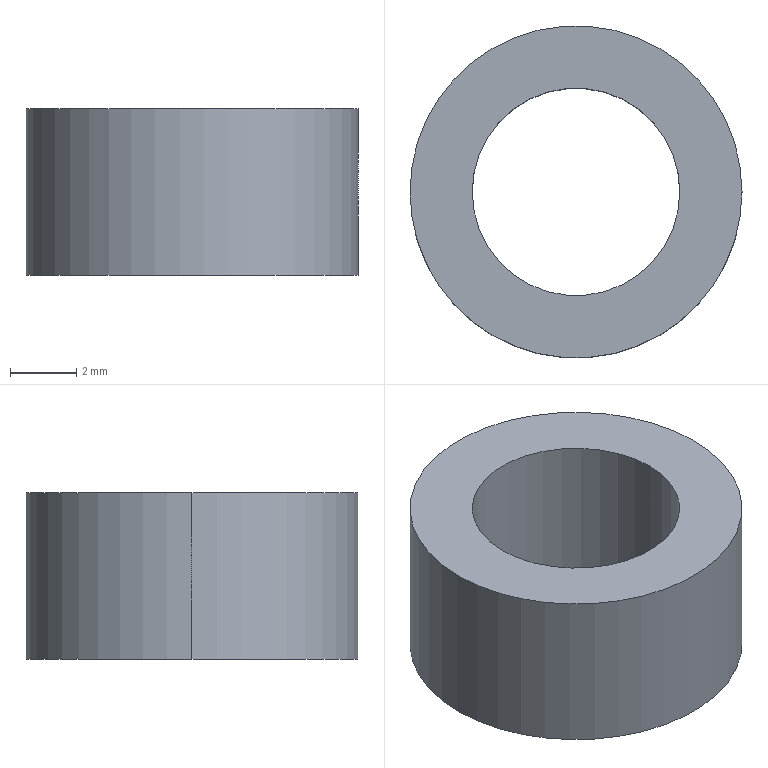Part | SolidWorks | features Extrusion 1 | 1 solid | 6 faces | box 10 x 10 x 5 mm | volume 239.301 mm3 | cylinder 4 | plane 2 | commonest cylinder face diameters 6.25 x2 10 x2
STEP:
#1=CARTESIAN_POINT('',(-0.123,0.,0.1969));
#2=VERTEX_POINT('',#1);
#3=CARTESIAN_POINT('',(0.123,0.,0.1969));
#4=VERTEX_POINT('',#3);
#5=CARTESIAN_POINT('',(0.,0.,0.1969));
#6=DIRECTION('',(0.,0.,1.));
#7=DIRECTION('',(1.,0.,0.));
#8=AXIS2_PLACEMENT_3D('',#5,#6,#7);
#9=CIRCLE('',#8,0.123);
#10=EDGE_CURVE('',#2,#4,#9,.T.);
#11=ORIENTED_EDGE('',*,*,#10,.T.);
#12=CARTESIAN_POINT('',(0.123,0.,0.));
#13=VERTEX_POINT('',#12);
#14=CARTESIAN_POINT('',(0.123,0.,0.1969));
#15=DIRECTION('',(0.,0.,-1.));
#16=VECTOR('',#15,39.37);
#17=LINE('',#14,#16);
#18=EDGE_CURVE('',#4,#13,#17,.T.);
#19=ORIENTED_EDGE('',*,*,#18,.T.);
#20=CARTESIAN_POINT('',(-0.123,0.,0.));
#21=VERTEX_POINT('',#20);
#22=CARTESIAN_POINT('',(0.,0.,0.));
#23=DIRECTION('',(0.,0.,1.));
#24=DIRECTION('',(1.,0.,0.));
#25=AXIS2_PLACEMENT_3D('',#22,#23,#24);
#26=CIRCLE('',#25,0.123);
#27=EDGE_CURVE('',#21,#13,#26,.T.);
#28=ORIENTED_EDGE('',*,*,#27,.F.);
#29=CARTESIAN_POINT('',(-0.123,0.,0.1969));
#30=DIRECTION('',(0.,0.,-1.));
#31=VECTOR('',#30,39.37);
#32=LINE('',#29,#31);
#33=EDGE_CURVE('',#2,#21,#32,.T.);
#34=ORIENTED_EDGE('',*,*,#33,.F.);
#35=EDGE_LOOP('',(#11,#19,#28,#34));
#36=FACE_OUTER_BOUND('',#35,.T.);
#37=CARTESIAN_POINT('',(0.,0.,0.1969));
#38=DIRECTION('',(0.,0.,-1.));
#39=DIRECTION('',(-1.,0.,0.));
#40=AXIS2_PLACEMENT_3D('',#37,#38,#39);
#41=CYLINDRICAL_SURFACE('',#40,0.123);
#42=ADVANCED_FACE('',(#36),#41,.F.);
#43=CARTESIAN_POINT('',(0.1969,0.,0.1969));
#44=VERTEX_POINT('',#43);
#45=CARTESIAN_POINT('',(-0.1969,0.,0.1969));
#46=VERTEX_POINT('',#45);
#47=CARTESIAN_POINT('',(0.,0.,0.1969));
#48=DIRECTION('',(0.,0.,1.));
#49=DIRECTION('',(1.,0.,0.));
#50=AXIS2_PLACEMENT_3D('',#47,#48,#49);
#51=CIRCLE('',#50,0.1969);
#52=EDGE_CURVE('',#44,#46,#51,.T.);
#53=ORIENTED_EDGE('',*,*,#52,.F.);
#54=CARTESIAN_POINT('',(0.1969,0.,0.));
#55=VERTEX_POINT('',#54);
#56=CARTESIAN_POINT('',(0.1969,0.,0.1969));
#57=DIRECTION('',(0.,0.,-1.));
#58=VECTOR('',#57,39.37);
#59=LINE('',#56,#58);
#60=EDGE_CURVE('',#44,#55,#59,.T.);
#61=ORIENTED_EDGE('',*,*,#60,.T.);
#62=CARTESIAN_POINT('',(-0.1969,0.,0.));
#63=VERTEX_POINT('',#62);
#64=CARTESIAN_POINT('',(0.,0.,0.));
#65=DIRECTION('',(0.,0.,1.));
#66=DIRECTION('',(1.,0.,0.));
#67=AXIS2_PLACEMENT_3D('',#64,#65,#66);
#68=CIRCLE('',#67,0.1969);
#69=EDGE_CURVE('',#55,#63,#68,.T.);
#70=ORIENTED_EDGE('',*,*,#69,.T.);
#71=CARTESIAN_POINT('',(-0.1969,0.,0.1969));
#72=DIRECTION('',(0.,0.,-1.));
#73=VECTOR('',#72,39.37);
#74=LINE('',#71,#73);
#75=EDGE_CURVE('',#46,#63,#74,.T.);
#76=ORIENTED_EDGE('',*,*,#75,.F.);
#77=EDGE_LOOP('',(#53,#61,#70,#76));
#78=FACE_OUTER_BOUND('',#77,.T.);
#79=CARTESIAN_POINT('',(0.,0.,0.1969));
#80=DIRECTION('',(0.,0.,-1.));
#81=DIRECTION('',(-1.,0.,0.));
#82=AXIS2_PLACEMENT_3D('',#79,#80,#81);
#83=CYLINDRICAL_SURFACE('',#82,0.1969);
#84=ADVANCED_FACE('',(#78),#83,.T.);
#85=CARTESIAN_POINT('',(0.,0.,0.1969));
#86=DIRECTION('',(0.,0.,1.));
#87=DIRECTION('',(1.,0.,0.));
#88=AXIS2_PLACEMENT_3D('',#85,#86,#87);
#89=CIRCLE('',#88,0.1969);
#90=EDGE_CURVE('',#46,#44,#89,.T.);
#91=ORIENTED_EDGE('',*,*,#90,.T.);
#92=ORIENTED_EDGE('',*,*,#52,.T.);
#93=EDGE_LOOP('',(#91,#92));
#94=FACE_OUTER_BOUND('',#93,.T.);
#95=ORIENTED_EDGE('',*,*,#10,.F.);
#96=CARTESIAN_POINT('',(0.,0.,0.1969));
#97=DIRECTION('',(0.,0.,1.));
#98=DIRECTION('',(1.,0.,0.));
#99=AXIS2_PLACEMENT_3D('',#96,#97,#98);
#100=CIRCLE('',#99,0.123);
#101=EDGE_CURVE('',#4,#2,#100,.T.);
#102=ORIENTED_EDGE('',*,*,#101,.F.);
#103=EDGE_LOOP('',(#95,#102));
#104=FACE_BOUND('',#103,.T.);
#105=CARTESIAN_POINT('',(0.,0.,0.1969));
#106=DIRECTION('',(0.,0.,1.));
#107=DIRECTION('',(1.,0.,0.));
#108=AXIS2_PLACEMENT_3D('',#105,#106,#107);
#109=PLANE('',#108);
#110=ADVANCED_FACE('',(#94,#104),#109,.T.);
#111=CARTESIAN_POINT('',(0.,0.,0.));
#112=DIRECTION('',(0.,0.,1.));
#113=DIRECTION('',(1.,0.,0.));
#114=AXIS2_PLACEMENT_3D('',#111,#112,#113);
#115=CIRCLE('',#114,0.1969);
#116=EDGE_CURVE('',#63,#55,#115,.T.);
#117=ORIENTED_EDGE('',*,*,#116,.F.);
#118=ORIENTED_EDGE('',*,*,#69,.F.);
#119=EDGE_LOOP('',(#117,#118));
#120=FACE_OUTER_BOUND('',#119,.T.);
#121=ORIENTED_EDGE('',*,*,#27,.T.);
#122=CARTESIAN_POINT('',(0.,0.,0.));
#123=DIRECTION('',(0.,0.,1.));
#124=DIRECTION('',(1.,0.,0.));
#125=AXIS2_PLACEMENT_3D('',#122,#123,#124);
#126=CIRCLE('',#125,0.123);
#127=EDGE_CURVE('',#13,#21,#126,.T.);
#128=ORIENTED_EDGE('',*,*,#127,.T.);
#129=EDGE_LOOP('',(#121,#128));
#130=FACE_BOUND('',#129,.T.);
#131=CARTESIAN_POINT('',(0.,0.,0.));
#132=DIRECTION('',(0.,0.,1.));
#133=DIRECTION('',(1.,0.,0.));
#134=AXIS2_PLACEMENT_3D('',#131,#132,#133);
#135=PLANE('',#134);
#136=ADVANCED_FACE('',(#120,#130),#135,.F.);
#137=ORIENTED_EDGE('',*,*,#60,.F.);
#138=ORIENTED_EDGE('',*,*,#90,.F.);
#139=ORIENTED_EDGE('',*,*,#75,.T.);
#140=ORIENTED_EDGE('',*,*,#116,.T.);
#141=EDGE_LOOP('',(#137,#138,#139,#140));
#142=FACE_OUTER_BOUND('',#141,.T.);
#143=CARTESIAN_POINT('',(0.,0.,0.1969));
#144=DIRECTION('',(0.,0.,-1.));
#145=DIRECTION('',(-1.,0.,0.));
#146=AXIS2_PLACEMENT_3D('',#143,#144,#145);
#147=CYLINDRICAL_SURFACE('',#146,0.1969);
#148=ADVANCED_FACE('',(#142),#147,.T.);
#149=ORIENTED_EDGE('',*,*,#18,.F.);
#150=ORIENTED_EDGE('',*,*,#101,.T.);
#151=ORIENTED_EDGE('',*,*,#33,.T.);
#152=ORIENTED_EDGE('',*,*,#127,.F.);
#153=EDGE_LOOP('',(#149,#150,#151,#152));
#154=FACE_OUTER_BOUND('',#153,.T.);
#155=CARTESIAN_POINT('',(0.,0.,0.1969));
#156=DIRECTION('',(0.,0.,-1.));
#157=DIRECTION('',(-1.,0.,0.));
#158=AXIS2_PLACEMENT_3D('',#155,#156,#157);
#159=CYLINDRICAL_SURFACE('',#158,0.123);
#160=ADVANCED_FACE('',(#154),#159,.F.);
#161=CLOSED_SHELL('',(#42,#84,#110,#136,#148,#160));
#162=MANIFOLD_SOLID_BREP('',#161);
#163=CARTESIAN_POINT('',(0.,0.,0.));
#164=DIRECTION('',(0.,0.,1.));
#165=DIRECTION('',(1.,0.,0.));
#166=AXIS2_PLACEMENT_3D('',#163,#164,#165);
#167=(LENGTH_UNIT()NAMED_UNIT(*)SI_UNIT($,.METRE.));
#168=LENGTH_MEASURE_WITH_UNIT(LENGTH_MEASURE(0.0254),#167);
#169=DIMENSIONAL_EXPONENTS(1.,0.,0.,0.,0.,0.,0.);
#170=(CONVERSION_BASED_UNIT('INCH',#168)LENGTH_UNIT()NAMED_UNIT(#169));
#171=UNCERTAINTY_MEASURE_WITH_UNIT(LENGTH_MEASURE(0.00001),#170,'','');
#172=(NAMED_UNIT(*)PLANE_ANGLE_UNIT()SI_UNIT($,.RADIAN.));
#173=(NAMED_UNIT(*)SI_UNIT($,.STERADIAN.)SOLID_ANGLE_UNIT());
#174=(GEOMETRIC_REPRESENTATION_CONTEXT(3)GLOBAL_UNCERTAINTY_ASSIGNED_CONTEXT((#171))GLOBAL_UNIT_ASSIGNED_CONTEXT((#170,#172,#173))REPRESENTATION_CONTEXT('',''));
#175=ADVANCED_BREP_SHAPE_REPRESENTATION('',(#162,#166),#174);